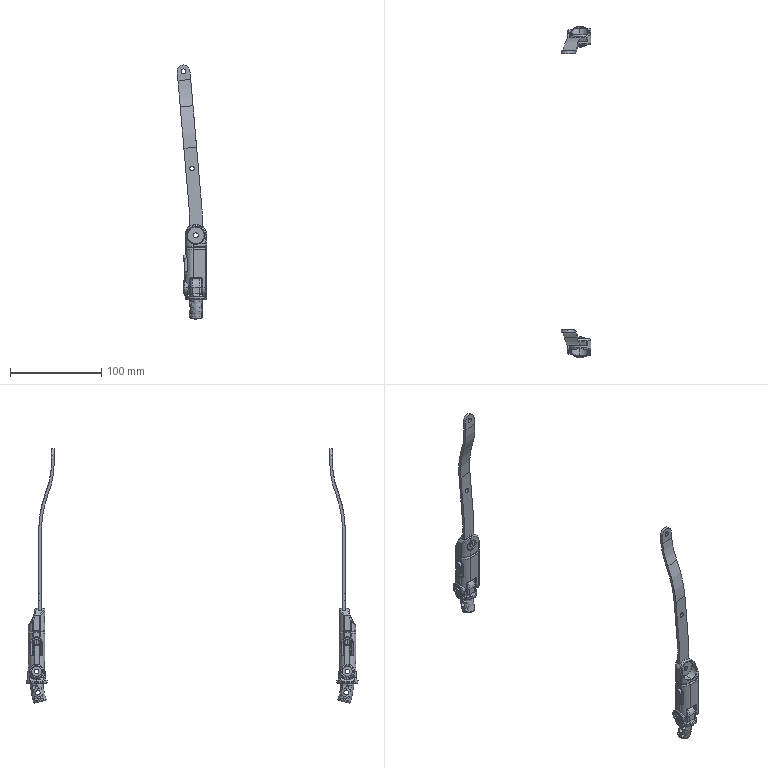Part | SolidWorks | features BaseBody 10 | 10 solids | 1068 faces | box 32.536 x 364.6 x 279.083 mm | volume 67490 mm3 | cylinder 497 | plane 272 | torus 149 | spline 114 | sphere 36 | commonest cylinder face diameters 2 x129 1 x104 5.2 x36 10.2 x32 3 x28 11 x14